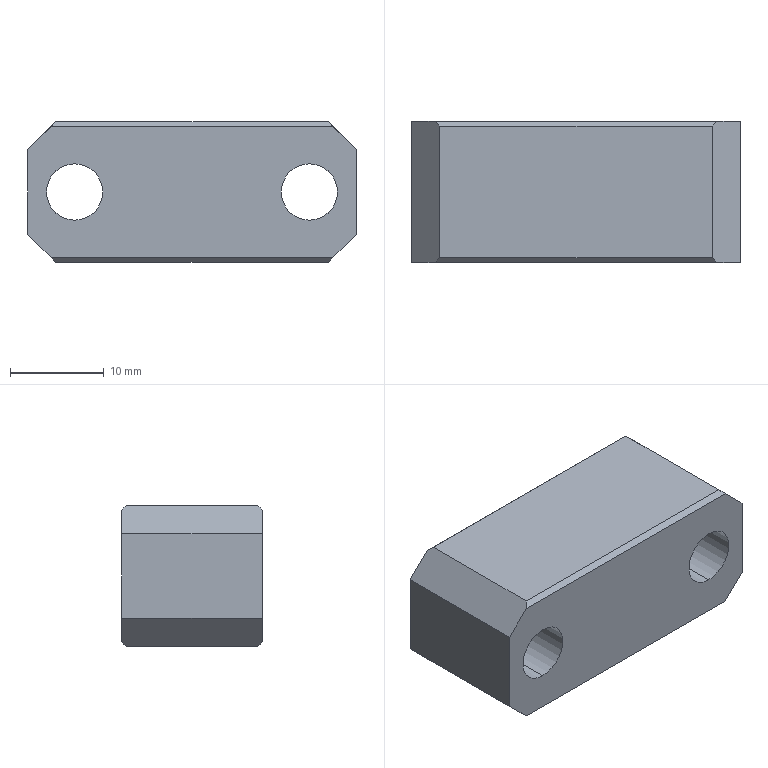Part | SolidWorks | features Chamfer 2, Extrusion 1, ICE 1 | 1 solid | 18 faces | box 35 x 15 x 15 mm | volume 6742 mm3 | plane 14 | cylinder 4 | commonest cylinder face diameters 6 x4
STEP:
#1=CARTESIAN_POINT('',(-55.073,0.,-12.635));
#2=VERTEX_POINT('',#1);
#3=CARTESIAN_POINT('',(-55.073,0.,-6.635));
#4=VERTEX_POINT('',#3);
#5=CARTESIAN_POINT('',(-55.073,0.,-9.635));
#6=DIRECTION('',(0.,1.,0.));
#7=DIRECTION('',(0.,0.,1.));
#8=AXIS2_PLACEMENT_3D('',#5,#6,#7);
#9=CIRCLE('',#8,3.);
#10=EDGE_CURVE('',#2,#4,#9,.T.);
#11=ORIENTED_EDGE('',*,*,#10,.F.);
#12=CARTESIAN_POINT('',(-55.073,15.,-12.635));
#13=VERTEX_POINT('',#12);
#14=CARTESIAN_POINT('',(-55.073,-0.7,-12.635));
#15=DIRECTION('',(0.,1.,0.));
#16=VECTOR('',#15,1000.);
#17=LINE('',#14,#16);
#18=EDGE_CURVE('',#2,#13,#17,.T.);
#19=ORIENTED_EDGE('',*,*,#18,.T.);
#20=CARTESIAN_POINT('',(-55.073,15.,-6.635));
#21=VERTEX_POINT('',#20);
#22=CARTESIAN_POINT('',(-55.073,15.,-9.635));
#23=DIRECTION('',(0.,1.,0.));
#24=DIRECTION('',(0.,0.,1.));
#25=AXIS2_PLACEMENT_3D('',#22,#23,#24);
#26=CIRCLE('',#25,3.);
#27=EDGE_CURVE('',#13,#21,#26,.T.);
#28=ORIENTED_EDGE('',*,*,#27,.T.);
#29=CARTESIAN_POINT('',(-55.073,-0.7,-6.635));
#30=DIRECTION('',(0.,1.,0.));
#31=VECTOR('',#30,1000.);
#32=LINE('',#29,#31);
#33=EDGE_CURVE('',#4,#21,#32,.T.);
#34=ORIENTED_EDGE('',*,*,#33,.F.);
#35=EDGE_LOOP('',(#11,#19,#28,#34));
#36=FACE_OUTER_BOUND('',#35,.T.);
#37=CARTESIAN_POINT('',(-55.073,-0.7,-9.635));
#38=DIRECTION('',(0.,1.,0.));
#39=DIRECTION('',(0.,0.,1.));
#40=AXIS2_PLACEMENT_3D('',#37,#38,#39);
#41=CYLINDRICAL_SURFACE('',#40,3.);
#42=ADVANCED_FACE('',(#36),#41,.F.);
#43=CARTESIAN_POINT('',(-80.073,0.,-12.635));
#44=VERTEX_POINT('',#43);
#45=CARTESIAN_POINT('',(-80.073,0.,-6.635));
#46=VERTEX_POINT('',#45);
#47=CARTESIAN_POINT('',(-80.073,0.,-9.635));
#48=DIRECTION('',(0.,1.,0.));
#49=DIRECTION('',(0.,0.,1.));
#50=AXIS2_PLACEMENT_3D('',#47,#48,#49);
#51=CIRCLE('',#50,3.);
#52=EDGE_CURVE('',#44,#46,#51,.T.);
#53=ORIENTED_EDGE('',*,*,#52,.F.);
#54=CARTESIAN_POINT('',(-80.073,15.,-12.635));
#55=VERTEX_POINT('',#54);
#56=CARTESIAN_POINT('',(-80.073,-0.7,-12.635));
#57=DIRECTION('',(0.,1.,0.));
#58=VECTOR('',#57,1000.);
#59=LINE('',#56,#58);
#60=EDGE_CURVE('',#44,#55,#59,.T.);
#61=ORIENTED_EDGE('',*,*,#60,.T.);
#62=CARTESIAN_POINT('',(-80.073,15.,-6.635));
#63=VERTEX_POINT('',#62);
#64=CARTESIAN_POINT('',(-80.073,15.,-9.635));
#65=DIRECTION('',(0.,1.,0.));
#66=DIRECTION('',(0.,0.,1.));
#67=AXIS2_PLACEMENT_3D('',#64,#65,#66);
#68=CIRCLE('',#67,3.);
#69=EDGE_CURVE('',#55,#63,#68,.T.);
#70=ORIENTED_EDGE('',*,*,#69,.T.);
#71=CARTESIAN_POINT('',(-80.073,-0.7,-6.635));
#72=DIRECTION('',(0.,1.,0.));
#73=VECTOR('',#72,1000.);
#74=LINE('',#71,#73);
#75=EDGE_CURVE('',#46,#63,#74,.T.);
#76=ORIENTED_EDGE('',*,*,#75,.F.);
#77=EDGE_LOOP('',(#53,#61,#70,#76));
#78=FACE_OUTER_BOUND('',#77,.T.);
#79=CARTESIAN_POINT('',(-80.073,-0.7,-9.635));
#80=DIRECTION('',(0.,1.,0.));
#81=DIRECTION('',(0.,0.,1.));
#82=AXIS2_PLACEMENT_3D('',#79,#80,#81);
#83=CYLINDRICAL_SURFACE('',#82,3.);
#84=ADVANCED_FACE('',(#78),#83,.F.);
#85=CARTESIAN_POINT('',(-85.073,0.,-14.135));
#86=VERTEX_POINT('',#85);
#87=CARTESIAN_POINT('',(-85.073,0.,-5.135));
#88=VERTEX_POINT('',#87);
#89=CARTESIAN_POINT('',(-85.073,0.,-17.135));
#90=DIRECTION('',(0.,0.,1.));
#91=VECTOR('',#90,1000.);
#92=LINE('',#89,#91);
#93=EDGE_CURVE('',#86,#88,#92,.T.);
#94=ORIENTED_EDGE('',*,*,#93,.T.);
#95=CARTESIAN_POINT('',(-85.073,15.,-5.135));
#96=VERTEX_POINT('',#95);
#97=CARTESIAN_POINT('',(-85.073,15.,-5.135));
#98=DIRECTION('',(0.,1.,0.));
#99=VECTOR('',#98,1000.);
#100=LINE('',#97,#99);
#101=EDGE_CURVE('',#88,#96,#100,.T.);
#102=ORIENTED_EDGE('',*,*,#101,.T.);
#103=CARTESIAN_POINT('',(-85.073,15.,-14.135));
#104=VERTEX_POINT('',#103);
#105=CARTESIAN_POINT('',(-85.073,15.,-17.135));
#106=DIRECTION('',(0.,0.,1.));
#107=VECTOR('',#106,1000.);
#108=LINE('',#105,#107);
#109=EDGE_CURVE('',#104,#96,#108,.T.);
#110=ORIENTED_EDGE('',*,*,#109,.F.);
#111=CARTESIAN_POINT('',(-85.073,15.,-14.135));
#112=DIRECTION('',(0.,-1.,0.));
#113=VECTOR('',#112,1000.);
#114=LINE('',#111,#113);
#115=EDGE_CURVE('',#104,#86,#114,.T.);
#116=ORIENTED_EDGE('',*,*,#115,.T.);
#117=EDGE_LOOP('',(#94,#102,#110,#116));
#118=FACE_OUTER_BOUND('',#117,.T.);
#119=CARTESIAN_POINT('',(-85.073,15.,-17.135));
#120=DIRECTION('',(1.,0.,0.));
#121=DIRECTION('',(0.,0.,-1.));
#122=AXIS2_PLACEMENT_3D('',#119,#120,#121);
#123=PLANE('',#122);
#124=ADVANCED_FACE('',(#118),#123,.F.);
#125=CARTESIAN_POINT('',(-82.073,14.5,-2.135));
#126=VERTEX_POINT('',#125);
#127=CARTESIAN_POINT('',(-82.073,0.5,-2.135));
#128=VERTEX_POINT('',#127);
#129=CARTESIAN_POINT('',(-82.073,15.,-2.135));
#130=DIRECTION('',(0.,-1.,0.));
#131=VECTOR('',#130,1000.);
#132=LINE('',#129,#131);
#133=EDGE_CURVE('',#126,#128,#132,.T.);
#134=ORIENTED_EDGE('',*,*,#133,.T.);
#135=CARTESIAN_POINT('',(-53.073,0.5,-2.135));
#136=VERTEX_POINT('',#135);
#137=CARTESIAN_POINT('',(-85.073,0.5,-2.135));
#138=DIRECTION('',(1.,0.,0.));
#139=VECTOR('',#138,1000.);
#140=LINE('',#137,#139);
#141=EDGE_CURVE('',#128,#136,#140,.T.);
#142=ORIENTED_EDGE('',*,*,#141,.T.);
#143=CARTESIAN_POINT('',(-53.073,14.5,-2.135));
#144=VERTEX_POINT('',#143);
#145=CARTESIAN_POINT('',(-53.073,15.,-2.135));
#146=DIRECTION('',(0.,1.,0.));
#147=VECTOR('',#146,1000.);
#148=LINE('',#145,#147);
#149=EDGE_CURVE('',#136,#144,#148,.T.);
#150=ORIENTED_EDGE('',*,*,#149,.T.);
#151=CARTESIAN_POINT('',(-82.073,14.5,-2.135));
#152=DIRECTION('',(-1.,0.,0.));
#153=VECTOR('',#152,1000.);
#154=LINE('',#151,#153);
#155=EDGE_CURVE('',#144,#126,#154,.T.);
#156=ORIENTED_EDGE('',*,*,#155,.T.);
#157=EDGE_LOOP('',(#134,#142,#150,#156));
#158=FACE_OUTER_BOUND('',#157,.T.);
#159=CARTESIAN_POINT('',(-85.073,15.,-2.135));
#160=DIRECTION('',(0.,0.,-1.));
#161=DIRECTION('',(-1.,0.,0.));
#162=AXIS2_PLACEMENT_3D('',#159,#160,#161);
#163=PLANE('',#162);
#164=ADVANCED_FACE('',(#158),#163,.F.);
#165=CARTESIAN_POINT('',(-50.073,15.,-5.135));
#166=VERTEX_POINT('',#165);
#167=CARTESIAN_POINT('',(-50.073,15.,-14.135));
#168=VERTEX_POINT('',#167);
#169=CARTESIAN_POINT('',(-50.073,15.,-17.135));
#170=DIRECTION('',(0.,0.,-1.));
#171=VECTOR('',#170,1000.);
#172=LINE('',#169,#171);
#173=EDGE_CURVE('',#166,#168,#172,.T.);
#174=ORIENTED_EDGE('',*,*,#173,.F.);
#175=CARTESIAN_POINT('',(-50.073,0.,-5.135));
#176=VERTEX_POINT('',#175);
#177=CARTESIAN_POINT('',(-50.073,15.,-5.135));
#178=DIRECTION('',(0.,-1.,0.));
#179=VECTOR('',#178,1000.);
#180=LINE('',#177,#179);
#181=EDGE_CURVE('',#166,#176,#180,.T.);
#182=ORIENTED_EDGE('',*,*,#181,.T.);
#183=CARTESIAN_POINT('',(-50.073,0.,-14.135));
#184=VERTEX_POINT('',#183);
#185=CARTESIAN_POINT('',(-50.073,0.,-17.135));
#186=DIRECTION('',(0.,0.,-1.));
#187=VECTOR('',#186,1000.);
#188=LINE('',#185,#187);
#189=EDGE_CURVE('',#176,#184,#188,.T.);
#190=ORIENTED_EDGE('',*,*,#189,.T.);
#191=CARTESIAN_POINT('',(-50.073,15.,-14.135));
#192=DIRECTION('',(0.,1.,0.));
#193=VECTOR('',#192,1000.);
#194=LINE('',#191,#193);
#195=EDGE_CURVE('',#184,#168,#194,.T.);
#196=ORIENTED_EDGE('',*,*,#195,.T.);
#197=EDGE_LOOP('',(#174,#182,#190,#196));
#198=FACE_OUTER_BOUND('',#197,.T.);
#199=CARTESIAN_POINT('',(-50.073,15.,-17.135));
#200=DIRECTION('',(-1.,0.,0.));
#201=DIRECTION('',(0.,0.,1.));
#202=AXIS2_PLACEMENT_3D('',#199,#200,#201);
#203=PLANE('',#202);
#204=ADVANCED_FACE('',(#198),#203,.F.);
#205=CARTESIAN_POINT('',(-53.073,14.5,-17.135));
#206=VERTEX_POINT('',#205);
#207=CARTESIAN_POINT('',(-53.073,0.5,-17.135));
#208=VERTEX_POINT('',#207);
#209=CARTESIAN_POINT('',(-53.073,15.,-17.135));
#210=DIRECTION('',(0.,-1.,0.));
#211=VECTOR('',#210,1000.);
#212=LINE('',#209,#211);
#213=EDGE_CURVE('',#206,#208,#212,.T.);
#214=ORIENTED_EDGE('',*,*,#213,.T.);
#215=CARTESIAN_POINT('',(-82.073,0.5,-17.135));
#216=VERTEX_POINT('',#215);
#217=CARTESIAN_POINT('',(-85.073,0.5,-17.135));
#218=DIRECTION('',(-1.,0.,0.));
#219=VECTOR('',#218,1000.);
#220=LINE('',#217,#219);
#221=EDGE_CURVE('',#208,#216,#220,.T.);
#222=ORIENTED_EDGE('',*,*,#221,.T.);
#223=CARTESIAN_POINT('',(-82.073,14.5,-17.135));
#224=VERTEX_POINT('',#223);
#225=CARTESIAN_POINT('',(-82.073,15.,-17.135));
#226=DIRECTION('',(0.,1.,0.));
#227=VECTOR('',#226,1000.);
#228=LINE('',#225,#227);
#229=EDGE_CURVE('',#216,#224,#228,.T.);
#230=ORIENTED_EDGE('',*,*,#229,.T.);
#231=CARTESIAN_POINT('',(-53.073,14.5,-17.135));
#232=DIRECTION('',(1.,0.,0.));
#233=VECTOR('',#232,1000.);
#234=LINE('',#231,#233);
#235=EDGE_CURVE('',#224,#206,#234,.T.);
#236=ORIENTED_EDGE('',*,*,#235,.T.);
#237=EDGE_LOOP('',(#214,#222,#230,#236));
#238=FACE_OUTER_BOUND('',#237,.T.);
#239=CARTESIAN_POINT('',(-85.073,15.,-17.135));
#240=DIRECTION('',(0.,0.,1.));
#241=DIRECTION('',(1.,0.,0.));
#242=AXIS2_PLACEMENT_3D('',#239,#240,#241);
#243=PLANE('',#242);
#244=ADVANCED_FACE('',(#238),#243,.F.);
#245=CARTESIAN_POINT('',(-55.073,15.,-9.635));
#246=DIRECTION('',(0.,1.,0.));
#247=DIRECTION('',(0.,0.,1.));
#248=AXIS2_PLACEMENT_3D('',#245,#246,#247);
#249=CIRCLE('',#248,3.);
#250=EDGE_CURVE('',#21,#13,#249,.T.);
#251=ORIENTED_EDGE('',*,*,#250,.F.);
#252=ORIENTED_EDGE('',*,*,#27,.F.);
#253=EDGE_LOOP('',(#251,#252));
#254=FACE_BOUND('',#253,.T.);
#255=CARTESIAN_POINT('',(-80.073,15.,-9.635));
#256=DIRECTION('',(0.,1.,0.));
#257=DIRECTION('',(0.,0.,1.));
#258=AXIS2_PLACEMENT_3D('',#255,#256,#257);
#259=CIRCLE('',#258,3.);
#260=EDGE_CURVE('',#63,#55,#259,.T.);
#261=ORIENTED_EDGE('',*,*,#260,.F.);
#262=ORIENTED_EDGE('',*,*,#69,.F.);
#263=EDGE_LOOP('',(#261,#262));
#264=FACE_BOUND('',#263,.T.);
#265=CARTESIAN_POINT('',(-82.573,15.,-2.635));
#266=VERTEX_POINT('',#265);
#267=CARTESIAN_POINT('',(-83.573,15.,-3.635));
#268=DIRECTION('',(0.7071,0.,0.7071));
#269=VECTOR('',#268,1000.);
#270=LINE('',#267,#269);
#271=EDGE_CURVE('',#96,#266,#270,.T.);
#272=ORIENTED_EDGE('',*,*,#271,.T.);
#273=CARTESIAN_POINT('',(-52.573,15.,-2.635));
#274=VERTEX_POINT('',#273);
#275=CARTESIAN_POINT('',(-53.073,15.,-2.635));
#276=DIRECTION('',(1.,0.,0.));
#277=VECTOR('',#276,1000.);
#278=LINE('',#275,#277);
#279=EDGE_CURVE('',#266,#274,#278,.T.);
#280=ORIENTED_EDGE('',*,*,#279,.T.);
#281=CARTESIAN_POINT('',(-69.073,15.,13.865));
#282=DIRECTION('',(0.7071,0.,-0.7071));
#283=VECTOR('',#282,1000.);
#284=LINE('',#281,#283);
#285=EDGE_CURVE('',#274,#166,#284,.T.);
#286=ORIENTED_EDGE('',*,*,#285,.T.);
#287=ORIENTED_EDGE('',*,*,#173,.T.);
#288=CARTESIAN_POINT('',(-52.573,15.,-16.635));
#289=VERTEX_POINT('',#288);
#290=CARTESIAN_POINT('',(-61.573,15.,-25.635));
#291=DIRECTION('',(-0.7071,0.,-0.7071));
#292=VECTOR('',#291,1000.);
#293=LINE('',#290,#292);
#294=EDGE_CURVE('',#168,#289,#293,.T.);
#295=ORIENTED_EDGE('',*,*,#294,.T.);
#296=CARTESIAN_POINT('',(-82.573,15.,-16.635));
#297=VERTEX_POINT('',#296);
#298=CARTESIAN_POINT('',(-82.073,15.,-16.635));
#299=DIRECTION('',(-1.,0.,0.));
#300=VECTOR('',#299,1000.);
#301=LINE('',#298,#300);
#302=EDGE_CURVE('',#289,#297,#301,.T.);
#303=ORIENTED_EDGE('',*,*,#302,.T.);
#304=CARTESIAN_POINT('',(-91.073,15.,-8.135));
#305=DIRECTION('',(-0.7071,0.,0.7071));
#306=VECTOR('',#305,1000.);
#307=LINE('',#304,#306);
#308=EDGE_CURVE('',#297,#104,#307,.T.);
#309=ORIENTED_EDGE('',*,*,#308,.T.);
#310=ORIENTED_EDGE('',*,*,#109,.T.);
#311=EDGE_LOOP('',(#272,#280,#286,#287,#295,#303,#309,#310));
#312=FACE_OUTER_BOUND('',#311,.T.);
#313=CARTESIAN_POINT('',(-85.073,15.,-2.135));
#314=DIRECTION('',(0.,1.,0.));
#315=DIRECTION('',(0.,0.,1.));
#316=AXIS2_PLACEMENT_3D('',#313,#314,#315);
#317=PLANE('',#316);
#318=ADVANCED_FACE('',(#254,#264,#312),#317,.T.);
#319=CARTESIAN_POINT('',(-55.073,0.,-9.635));
#320=DIRECTION('',(0.,1.,0.));
#321=DIRECTION('',(0.,0.,1.));
#322=AXIS2_PLACEMENT_3D('',#319,#320,#321);
#323=CIRCLE('',#322,3.);
#324=EDGE_CURVE('',#4,#2,#323,.T.);
#325=ORIENTED_EDGE('',*,*,#324,.T.);
#326=ORIENTED_EDGE('',*,*,#10,.T.);
#327=EDGE_LOOP('',(#325,#326));
#328=FACE_BOUND('',#327,.T.);
#329=CARTESIAN_POINT('',(-80.073,0.,-9.635));
#330=DIRECTION('',(0.,1.,0.));
#331=DIRECTION('',(0.,0.,1.));
#332=AXIS2_PLACEMENT_3D('',#329,#330,#331);
#333=CIRCLE('',#332,3.);
#334=EDGE_CURVE('',#46,#44,#333,.T.);
#335=ORIENTED_EDGE('',*,*,#334,.T.);
#336=ORIENTED_EDGE('',*,*,#52,.T.);
#337=EDGE_LOOP('',(#335,#336));
#338=FACE_BOUND('',#337,.T.);
#339=CARTESIAN_POINT('',(-82.573,0.,-16.635));
#340=VERTEX_POINT('',#339);
#341=CARTESIAN_POINT('',(-85.073,0.,-14.135));
#342=DIRECTION('',(0.7071,0.,-0.7071));
#343=VECTOR('',#342,1000.);
#344=LINE('',#341,#343);
#345=EDGE_CURVE('',#86,#340,#344,.T.);
#346=ORIENTED_EDGE('',*,*,#345,.T.);
#347=CARTESIAN_POINT('',(-52.573,0.,-16.635));
#348=VERTEX_POINT('',#347);
#349=CARTESIAN_POINT('',(-85.073,0.,-16.635));
#350=DIRECTION('',(1.,0.,0.));
#351=VECTOR('',#350,1000.);
#352=LINE('',#349,#351);
#353=EDGE_CURVE('',#340,#348,#352,.T.);
#354=ORIENTED_EDGE('',*,*,#353,.T.);
#355=CARTESIAN_POINT('',(-53.073,0.,-17.135));
#356=DIRECTION('',(0.7071,0.,0.7071));
#357=VECTOR('',#356,1000.);
#358=LINE('',#355,#357);
#359=EDGE_CURVE('',#348,#184,#358,.T.);
#360=ORIENTED_EDGE('',*,*,#359,.T.);
#361=ORIENTED_EDGE('',*,*,#189,.F.);
#362=CARTESIAN_POINT('',(-52.573,0.,-2.635));
#363=VERTEX_POINT('',#362);
#364=CARTESIAN_POINT('',(-50.073,0.,-5.135));
#365=DIRECTION('',(-0.7071,0.,0.7071));
#366=VECTOR('',#365,1000.);
#367=LINE('',#364,#366);
#368=EDGE_CURVE('',#176,#363,#367,.T.);
#369=ORIENTED_EDGE('',*,*,#368,.T.);
#370=CARTESIAN_POINT('',(-82.573,0.,-2.635));
#371=VERTEX_POINT('',#370);
#372=CARTESIAN_POINT('',(-85.073,0.,-2.635));
#373=DIRECTION('',(-1.,0.,0.));
#374=VECTOR('',#373,1000.);
#375=LINE('',#372,#374);
#376=EDGE_CURVE('',#363,#371,#375,.T.);
#377=ORIENTED_EDGE('',*,*,#376,.T.);
#378=CARTESIAN_POINT('',(-82.073,0.,-2.135));
#379=DIRECTION('',(-0.7071,0.,-0.7071));
#380=VECTOR('',#379,1000.);
#381=LINE('',#378,#380);
#382=EDGE_CURVE('',#371,#88,#381,.T.);
#383=ORIENTED_EDGE('',*,*,#382,.T.);
#384=ORIENTED_EDGE('',*,*,#93,.F.);
#385=EDGE_LOOP('',(#346,#354,#360,#361,#369,#377,#383,#384));
#386=FACE_OUTER_BOUND('',#385,.T.);
#387=CARTESIAN_POINT('',(-85.073,0.,-2.135));
#388=DIRECTION('',(0.,1.,0.));
#389=DIRECTION('',(0.,0.,1.));
#390=AXIS2_PLACEMENT_3D('',#387,#388,#389);
#391=PLANE('',#390);
#392=ADVANCED_FACE('',(#328,#338,#386),#391,.F.);
#393=ORIENTED_EDGE('',*,*,#60,.F.);
#394=ORIENTED_EDGE('',*,*,#334,.F.);
#395=ORIENTED_EDGE('',*,*,#75,.T.);
#396=ORIENTED_EDGE('',*,*,#260,.T.);
#397=EDGE_LOOP('',(#393,#394,#395,#396));
#398=FACE_OUTER_BOUND('',#397,.T.);
#399=CARTESIAN_POINT('',(-80.073,-0.7,-9.635));
#400=DIRECTION('',(0.,1.,0.));
#401=DIRECTION('',(0.,0.,1.));
#402=AXIS2_PLACEMENT_3D('',#399,#400,#401);
#403=CYLINDRICAL_SURFACE('',#402,3.);
#404=ADVANCED_FACE('',(#398),#403,.F.);
#405=ORIENTED_EDGE('',*,*,#18,.F.);
#406=ORIENTED_EDGE('',*,*,#324,.F.);
#407=ORIENTED_EDGE('',*,*,#33,.T.);
#408=ORIENTED_EDGE('',*,*,#250,.T.);
#409=EDGE_LOOP('',(#405,#406,#407,#408));
#410=FACE_OUTER_BOUND('',#409,.T.);
#411=CARTESIAN_POINT('',(-55.073,-0.7,-9.635));
#412=DIRECTION('',(0.,1.,0.));
#413=DIRECTION('',(0.,0.,1.));
#414=AXIS2_PLACEMENT_3D('',#411,#412,#413);
#415=CYLINDRICAL_SURFACE('',#414,3.);
#416=ADVANCED_FACE('',(#410),#415,.F.);
#417=ORIENTED_EDGE('',*,*,#149,.F.);
#418=CARTESIAN_POINT('',(-55.907,3.333,0.6985));
#419=DIRECTION('',(0.5774,-0.5774,-0.5774));
#420=VECTOR('',#419,1000.);
#421=LINE('',#418,#420);
#422=EDGE_CURVE('',#136,#363,#421,.T.);
#423=ORIENTED_EDGE('',*,*,#422,.T.);
#424=ORIENTED_EDGE('',*,*,#368,.F.);
#425=ORIENTED_EDGE('',*,*,#181,.F.);
#426=ORIENTED_EDGE('',*,*,#285,.F.);
#427=CARTESIAN_POINT('',(-50.907,16.667,-4.302));
#428=DIRECTION('',(-0.5774,-0.5774,0.5774));
#429=VECTOR('',#428,1000.);
#430=LINE('',#427,#429);
#431=EDGE_CURVE('',#274,#144,#430,.T.);
#432=ORIENTED_EDGE('',*,*,#431,.T.);
#433=EDGE_LOOP('',(#417,#423,#424,#425,#426,#432));
#434=FACE_OUTER_BOUND('',#433,.T.);
#435=CARTESIAN_POINT('',(-50.073,15.,-5.135));
#436=DIRECTION('',(-0.7071,0.,-0.7071));
#437=DIRECTION('',(-0.7071,0.,0.7071));
#438=AXIS2_PLACEMENT_3D('',#435,#436,#437);
#439=PLANE('',#438);
#440=ADVANCED_FACE('',(#434),#439,.F.);
#441=ORIENTED_EDGE('',*,*,#359,.F.);
#442=CARTESIAN_POINT('',(-57.907,5.333,-21.968));
#443=DIRECTION('',(-0.5774,0.5774,-0.5774));
#444=VECTOR('',#443,1000.);
#445=LINE('',#442,#444);
#446=EDGE_CURVE('',#348,#208,#445,.T.);
#447=ORIENTED_EDGE('',*,*,#446,.T.);
#448=ORIENTED_EDGE('',*,*,#213,.F.);
#449=CARTESIAN_POINT('',(-52.907,14.667,-16.968));
#450=DIRECTION('',(0.5774,0.5774,0.5774));
#451=VECTOR('',#450,1000.);
#452=LINE('',#449,#451);
#453=EDGE_CURVE('',#206,#289,#452,.T.);
#454=ORIENTED_EDGE('',*,*,#453,.T.);
#455=ORIENTED_EDGE('',*,*,#294,.F.);
#456=ORIENTED_EDGE('',*,*,#195,.F.);
#457=EDGE_LOOP('',(#441,#447,#448,#454,#455,#456));
#458=FACE_OUTER_BOUND('',#457,.T.);
#459=CARTESIAN_POINT('',(-53.073,15.,-17.135));
#460=DIRECTION('',(-0.7071,0.,0.7071));
#461=DIRECTION('',(0.7071,0.,0.7071));
#462=AXIS2_PLACEMENT_3D('',#459,#460,#461);
#463=PLANE('',#462);
#464=ADVANCED_FACE('',(#458),#463,.F.);
#465=ORIENTED_EDGE('',*,*,#382,.F.);
#466=CARTESIAN_POINT('',(-77.24,5.333,2.698));
#467=DIRECTION('',(0.5774,0.5774,0.5774));
#468=VECTOR('',#467,1000.);
#469=LINE('',#466,#468);
#470=EDGE_CURVE('',#371,#128,#469,.T.);
#471=ORIENTED_EDGE('',*,*,#470,.T.);
#472=ORIENTED_EDGE('',*,*,#133,.F.);
#473=CARTESIAN_POINT('',(-82.24,14.667,-2.302));
#474=DIRECTION('',(-0.5774,0.5774,-0.5774));
#475=VECTOR('',#474,1000.);
#476=LINE('',#473,#475);
#477=EDGE_CURVE('',#126,#266,#476,.T.);
#478=ORIENTED_EDGE('',*,*,#477,.T.);
#479=ORIENTED_EDGE('',*,*,#271,.F.);
#480=ORIENTED_EDGE('',*,*,#101,.F.);
#481=EDGE_LOOP('',(#465,#471,#472,#478,#479,#480));
#482=FACE_OUTER_BOUND('',#481,.T.);
#483=CARTESIAN_POINT('',(-82.073,15.,-2.135));
#484=DIRECTION('',(0.7071,0.,-0.7071));
#485=DIRECTION('',(-0.7071,0.,-0.7071));
#486=AXIS2_PLACEMENT_3D('',#483,#484,#485);
#487=PLANE('',#486);
#488=ADVANCED_FACE('',(#482),#487,.F.);
#489=ORIENTED_EDGE('',*,*,#229,.F.);
#490=CARTESIAN_POINT('',(-79.24,3.333,-19.968));
#491=DIRECTION('',(-0.5774,-0.5774,0.5774));
#492=VECTOR('',#491,1000.);
#493=LINE('',#490,#492);
#494=EDGE_CURVE('',#216,#340,#493,.T.);
#495=ORIENTED_EDGE('',*,*,#494,.T.);
#496=ORIENTED_EDGE('',*,*,#345,.F.);
#497=ORIENTED_EDGE('',*,*,#115,.F.);
#498=ORIENTED_EDGE('',*,*,#308,.F.);
#499=CARTESIAN_POINT('',(-84.24,16.667,-14.968));
#500=DIRECTION('',(0.5774,-0.5774,-0.5774));
#501=VECTOR('',#500,1000.);
#502=LINE('',#499,#501);
#503=EDGE_CURVE('',#297,#224,#502,.T.);
#504=ORIENTED_EDGE('',*,*,#503,.T.);
#505=EDGE_LOOP('',(#489,#495,#496,#497,#498,#504));
#506=FACE_OUTER_BOUND('',#505,.T.);
#507=CARTESIAN_POINT('',(-85.073,15.,-14.135));
#508=DIRECTION('',(0.7071,0.,0.7071));
#509=DIRECTION('',(0.7071,0.,-0.7071));
#510=AXIS2_PLACEMENT_3D('',#507,#508,#509);
#511=PLANE('',#510);
#512=ADVANCED_FACE('',(#506),#511,.F.);
#513=ORIENTED_EDGE('',*,*,#446,.F.);
#514=ORIENTED_EDGE('',*,*,#353,.F.);
#515=ORIENTED_EDGE('',*,*,#494,.F.);
#516=ORIENTED_EDGE('',*,*,#221,.F.);
#517=EDGE_LOOP('',(#513,#514,#515,#516));
#518=FACE_OUTER_BOUND('',#517,.T.);
#519=CARTESIAN_POINT('',(-85.073,0.5,-17.135));
#520=DIRECTION('',(0.,0.7071,0.7071));
#521=DIRECTION('',(-1.,0.,0.));
#522=AXIS2_PLACEMENT_3D('',#519,#520,#521);
#523=PLANE('',#522);
#524=ADVANCED_FACE('',(#518),#523,.F.);
#525=ORIENTED_EDGE('',*,*,#470,.F.);
#526=ORIENTED_EDGE('',*,*,#376,.F.);
#527=ORIENTED_EDGE('',*,*,#422,.F.);
#528=ORIENTED_EDGE('',*,*,#141,.F.);
#529=EDGE_LOOP('',(#525,#526,#527,#528));
#530=FACE_OUTER_BOUND('',#529,.T.);
#531=CARTESIAN_POINT('',(-85.073,0.5,-2.135));
#532=DIRECTION('',(0.,0.7071,-0.7071));
#533=DIRECTION('',(1.,0.,0.));
#534=AXIS2_PLACEMENT_3D('',#531,#532,#533);
#535=PLANE('',#534);
#536=ADVANCED_FACE('',(#530),#535,.F.);
#537=ORIENTED_EDGE('',*,*,#477,.F.);
#538=ORIENTED_EDGE('',*,*,#155,.F.);
#539=ORIENTED_EDGE('',*,*,#431,.F.);
#540=ORIENTED_EDGE('',*,*,#279,.F.);
#541=EDGE_LOOP('',(#537,#538,#539,#540));
#542=FACE_OUTER_BOUND('',#541,.T.);
#543=CARTESIAN_POINT('',(-85.073,15.,-2.635));
#544=DIRECTION('',(0.,0.7071,0.7071));
#545=DIRECTION('',(-1.,0.,0.));
#546=AXIS2_PLACEMENT_3D('',#543,#544,#545);
#547=PLANE('',#546);
#548=ADVANCED_FACE('',(#542),#547,.T.);
#549=ORIENTED_EDGE('',*,*,#453,.F.);
#550=ORIENTED_EDGE('',*,*,#235,.F.);
#551=ORIENTED_EDGE('',*,*,#503,.F.);
#552=ORIENTED_EDGE('',*,*,#302,.F.);
#553=EDGE_LOOP('',(#549,#550,#551,#552));
#554=FACE_OUTER_BOUND('',#553,.T.);
#555=CARTESIAN_POINT('',(-85.073,15.,-16.635));
#556=DIRECTION('',(0.,0.7071,-0.7071));
#557=DIRECTION('',(1.,0.,0.));
#558=AXIS2_PLACEMENT_3D('',#555,#556,#557);
#559=PLANE('',#558);
#560=ADVANCED_FACE('',(#554),#559,.T.);
#561=CLOSED_SHELL('',(#42,#84,#124,#164,#204,#244,#318,#392,#404,#416,#440,#464,#488,#512,#524,#536,#548,#560));
#562=MANIFOLD_SOLID_BREP('',#561);
#563=CARTESIAN_POINT('',(0.,0.,0.));
#564=DIRECTION('',(0.,0.,1.));
#565=DIRECTION('',(1.,0.,0.));
#566=AXIS2_PLACEMENT_3D('',#563,#564,#565);
#567=(LENGTH_UNIT()NAMED_UNIT(*)SI_UNIT(.MILLI.,.METRE.));
#568=UNCERTAINTY_MEASURE_WITH_UNIT(LENGTH_MEASURE(0.00001),#567,'','');
#569=(NAMED_UNIT(*)PLANE_ANGLE_UNIT()SI_UNIT($,.RADIAN.));
#570=(NAMED_UNIT(*)SI_UNIT($,.STERADIAN.)SOLID_ANGLE_UNIT());
#571=(GEOMETRIC_REPRESENTATION_CONTEXT(3)GLOBAL_UNCERTAINTY_ASSIGNED_CONTEXT((#568))GLOBAL_UNIT_ASSIGNED_CONTEXT((#567,#569,#570))REPRESENTATION_CONTEXT('',''));
#572=ADVANCED_BREP_SHAPE_REPRESENTATION('',(#562,#566),#571);